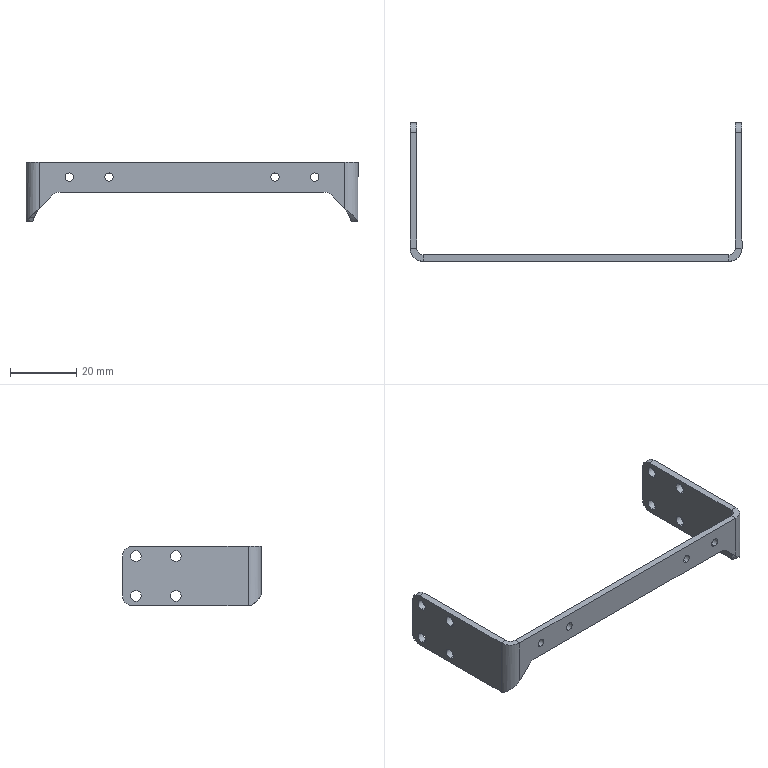Part | SolidWorks | features Fillet 1, FlatPattern 1, HoleWzd 1, SM3dBend 1, SMBaseFlange 1, SheetMetal 1 | 1 solid | 56 faces | box 100 x 41.788 x 18 mm | volume 4551 mm3 | cylinder 34 | plane 20 | spline 2 | commonest cylinder face diameters 3.2 x16 2.5 x8 6 x6 4 x2 8 x2